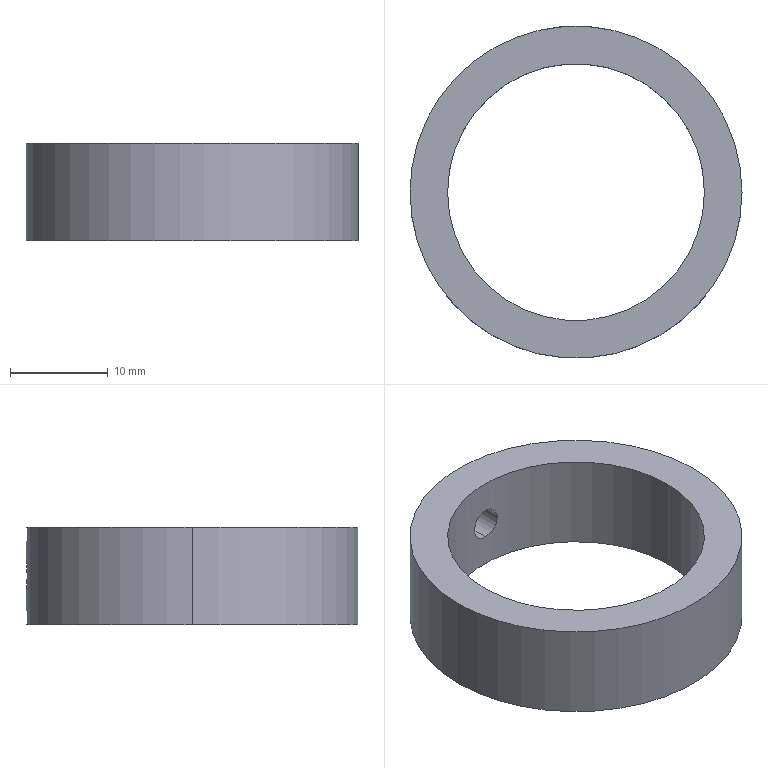Part | SolidWorks | features Extrusion 1, HoleWzd 1 | 1 solid | 8 faces | box 34 x 34 x 10 mm | volume 3614 mm3 | cylinder 6 | plane 2 | commonest cylinder face diameters 3.3 x2 26.3 x2 34 x2
STEP:
#1=CARTESIAN_POINT('',(0.,17.,1.65));
#2=VERTEX_POINT('',#1);
#3=CARTESIAN_POINT('',(0.,17.,-1.65));
#4=VERTEX_POINT('',#3);
#5=CARTESIAN_POINT('',(0.,17.,1.65));
#6=CARTESIAN_POINT('',(-0.2154,17.,1.65));
#7=CARTESIAN_POINT('',(-0.4326,16.996,1.607));
#8=CARTESIAN_POINT('',(-0.8297,16.981,1.442));
#9=CARTESIAN_POINT('',(-1.014,16.97,1.32));
#10=CARTESIAN_POINT('',(-1.242,16.955,1.092));
#11=CARTESIAN_POINT('',(-1.312,16.949,1.007));
#12=CARTESIAN_POINT('',(-1.432,16.94,0.8275));
#13=CARTESIAN_POINT('',(-1.482,16.935,0.7328));
#14=CARTESIAN_POINT('',(-1.565,16.928,0.5332));
#15=CARTESIAN_POINT('',(-1.597,16.925,0.4284));
#16=CARTESIAN_POINT('',(-1.639,16.921,0.2174));
#17=CARTESIAN_POINT('',(-1.65,16.92,0.1103));
#18=CARTESIAN_POINT('',(-1.65,16.92,-0.1077));
#19=CARTESIAN_POINT('',(-1.639,16.921,-0.2151));
#20=CARTESIAN_POINT('',(-1.598,16.925,-0.4261));
#21=CARTESIAN_POINT('',(-1.566,16.928,-0.5309));
#22=CARTESIAN_POINT('',(-1.483,16.935,-0.7308));
#23=CARTESIAN_POINT('',(-1.433,16.94,-0.8255));
#24=CARTESIAN_POINT('',(-1.313,16.949,-1.005));
#25=CARTESIAN_POINT('',(-1.244,16.955,-1.09));
#26=CARTESIAN_POINT('',(-1.016,16.97,-1.318));
#27=CARTESIAN_POINT('',(-0.8317,16.981,-1.441));
#28=CARTESIAN_POINT('',(-0.4348,16.996,-1.606));
#29=CARTESIAN_POINT('',(-0.2181,17.,-1.65));
#30=CARTESIAN_POINT('',(0.,17.,-1.65));
#31=B_SPLINE_CURVE_WITH_KNOTS('',3,(#5,#6,#7,#8,#9,#10,#11,#12,#13,#14,#15,#16,#17,#18,#19,#20,#21,#22,#23,#24,#25,#26,#27,#28,#29,#30),.UNSPECIFIED.,.F.,.F.,(4,2,2,2,2,2,2,2,2,2,2,2,4),(0.005162,0.005807,0.006452,0.006774,0.007097,0.007419,0.007742,0.008064,0.008387,0.00871,0.009032,0.009677,0.01032),.UNSPECIFIED.);
#32=EDGE_CURVE('',#2,#4,#31,.T.);
#33=ORIENTED_EDGE('',*,*,#32,.F.);
#34=CARTESIAN_POINT('',(0.,13.15,1.65));
#35=VERTEX_POINT('',#34);
#36=CARTESIAN_POINT('',(0.,0.,1.65));
#37=DIRECTION('',(0.,-1.,0.));
#38=VECTOR('',#37,1000.);
#39=LINE('',#36,#38);
#40=EDGE_CURVE('',#2,#35,#39,.T.);
#41=ORIENTED_EDGE('',*,*,#40,.T.);
#42=CARTESIAN_POINT('',(0.,13.15,-1.65));
#43=VERTEX_POINT('',#42);
#44=CARTESIAN_POINT('',(0.,13.15,1.65));
#45=CARTESIAN_POINT('',(-0.2154,13.15,1.65));
#46=CARTESIAN_POINT('',(-0.4327,13.144,1.607));
#47=CARTESIAN_POINT('',(-0.8299,13.125,1.442));
#48=CARTESIAN_POINT('',(-1.014,13.112,1.319));
#49=CARTESIAN_POINT('',(-1.242,13.091,1.092));
#50=CARTESIAN_POINT('',(-1.312,13.085,1.007));
#51=CARTESIAN_POINT('',(-1.431,13.072,0.8276));
#52=CARTESIAN_POINT('',(-1.482,13.066,0.733));
#53=CARTESIAN_POINT('',(-1.565,13.057,0.5333));
#54=CARTESIAN_POINT('',(-1.597,13.053,0.4285));
#55=CARTESIAN_POINT('',(-1.639,13.047,0.2176));
#56=CARTESIAN_POINT('',(-1.65,13.046,0.1103));
#57=CARTESIAN_POINT('',(-1.65,13.046,-0.1079));
#58=CARTESIAN_POINT('',(-1.639,13.047,-0.2152));
#59=CARTESIAN_POINT('',(-1.598,13.053,-0.4262));
#60=CARTESIAN_POINT('',(-1.566,13.056,-0.5311));
#61=CARTESIAN_POINT('',(-1.483,13.066,-0.7309));
#62=CARTESIAN_POINT('',(-1.433,13.072,-0.8256));
#63=CARTESIAN_POINT('',(-1.313,13.084,-1.005));
#64=CARTESIAN_POINT('',(-1.243,13.091,-1.09));
#65=CARTESIAN_POINT('',(-1.016,13.112,-1.318));
#66=CARTESIAN_POINT('',(-0.8318,13.125,-1.441));
#67=CARTESIAN_POINT('',(-0.435,13.144,-1.606));
#68=CARTESIAN_POINT('',(-0.2182,13.15,-1.65));
#69=CARTESIAN_POINT('',(0.,13.15,-1.65));
#70=B_SPLINE_CURVE_WITH_KNOTS('',3,(#44,#45,#46,#47,#48,#49,#50,#51,#52,#53,#54,#55,#56,#57,#58,#59,#60,#61,#62,#63,#64,#65,#66,#67,#68,#69),.UNSPECIFIED.,.F.,.F.,(4,2,2,2,2,2,2,2,2,2,2,2,4),(0.005164,0.005809,0.006454,0.006777,0.0071,0.007422,0.007745,0.008068,0.00839,0.008713,0.009036,0.009681,0.01033),.UNSPECIFIED.);
#71=EDGE_CURVE('',#35,#43,#70,.T.);
#72=ORIENTED_EDGE('',*,*,#71,.T.);
#73=CARTESIAN_POINT('',(0.,0.,-1.65));
#74=DIRECTION('',(0.,-1.,0.));
#75=VECTOR('',#74,1000.);
#76=LINE('',#73,#75);
#77=EDGE_CURVE('',#4,#43,#76,.T.);
#78=ORIENTED_EDGE('',*,*,#77,.F.);
#79=EDGE_LOOP('',(#33,#41,#72,#78));
#80=FACE_OUTER_BOUND('',#79,.T.);
#81=CARTESIAN_POINT('',(0.,0.,0.));
#82=DIRECTION('',(0.,-1.,0.));
#83=DIRECTION('',(0.,0.,-1.));
#84=AXIS2_PLACEMENT_3D('',#81,#82,#83);
#85=CYLINDRICAL_SURFACE('',#84,1.65);
#86=ADVANCED_FACE('',(#80),#85,.F.);
#87=CARTESIAN_POINT('',(-13.15,0.,5.));
#88=VERTEX_POINT('',#87);
#89=CARTESIAN_POINT('',(13.15,0.,5.));
#90=VERTEX_POINT('',#89);
#91=CARTESIAN_POINT('',(0.,0.,5.));
#92=DIRECTION('',(0.,0.,1.));
#93=DIRECTION('',(1.,0.,0.));
#94=AXIS2_PLACEMENT_3D('',#91,#92,#93);
#95=CIRCLE('',#94,13.15);
#96=EDGE_CURVE('',#88,#90,#95,.T.);
#97=ORIENTED_EDGE('',*,*,#96,.T.);
#98=CARTESIAN_POINT('',(13.15,0.,-5.));
#99=VERTEX_POINT('',#98);
#100=CARTESIAN_POINT('',(13.15,0.,5.));
#101=DIRECTION('',(0.,0.,-1.));
#102=VECTOR('',#101,1000.);
#103=LINE('',#100,#102);
#104=EDGE_CURVE('',#90,#99,#103,.T.);
#105=ORIENTED_EDGE('',*,*,#104,.T.);
#106=CARTESIAN_POINT('',(-13.15,0.,-5.));
#107=VERTEX_POINT('',#106);
#108=CARTESIAN_POINT('',(0.,0.,-5.));
#109=DIRECTION('',(0.,0.,1.));
#110=DIRECTION('',(1.,0.,0.));
#111=AXIS2_PLACEMENT_3D('',#108,#109,#110);
#112=CIRCLE('',#111,13.15);
#113=EDGE_CURVE('',#107,#99,#112,.T.);
#114=ORIENTED_EDGE('',*,*,#113,.F.);
#115=CARTESIAN_POINT('',(-13.15,0.,5.));
#116=DIRECTION('',(0.,0.,-1.));
#117=VECTOR('',#116,1000.);
#118=LINE('',#115,#117);
#119=EDGE_CURVE('',#88,#107,#118,.T.);
#120=ORIENTED_EDGE('',*,*,#119,.F.);
#121=EDGE_LOOP('',(#97,#105,#114,#120));
#122=FACE_OUTER_BOUND('',#121,.T.);
#123=CARTESIAN_POINT('',(0.,0.,5.));
#124=DIRECTION('',(0.,0.,-1.));
#125=DIRECTION('',(-1.,0.,0.));
#126=AXIS2_PLACEMENT_3D('',#123,#124,#125);
#127=CYLINDRICAL_SURFACE('',#126,13.15);
#128=ADVANCED_FACE('',(#122),#127,.F.);
#129=CARTESIAN_POINT('',(0.,17.,-1.65));
#130=CARTESIAN_POINT('',(0.1091,17.,-1.65));
#131=CARTESIAN_POINT('',(0.2163,16.999,-1.639));
#132=CARTESIAN_POINT('',(0.4273,16.995,-1.597));
#133=CARTESIAN_POINT('',(0.5322,16.992,-1.566));
#134=CARTESIAN_POINT('',(0.732,16.985,-1.483));
#135=CARTESIAN_POINT('',(0.8267,16.98,-1.432));
#136=CARTESIAN_POINT('',(1.006,16.97,-1.312));
#137=CARTESIAN_POINT('',(1.091,16.965,-1.243));
#138=CARTESIAN_POINT('',(1.319,16.949,-1.014));
#139=CARTESIAN_POINT('',(1.442,16.939,-0.8303));
#140=CARTESIAN_POINT('',(1.607,16.924,-0.4332));
#141=CARTESIAN_POINT('',(1.65,16.92,-0.216));
#142=CARTESIAN_POINT('',(1.65,16.92,0.1071));
#143=CARTESIAN_POINT('',(1.639,16.921,0.2165));
#144=CARTESIAN_POINT('',(1.597,16.925,0.4282));
#145=CARTESIAN_POINT('',(1.566,16.928,0.531));
#146=CARTESIAN_POINT('',(1.483,16.935,0.7309));
#147=CARTESIAN_POINT('',(1.432,16.94,0.8274));
#148=CARTESIAN_POINT('',(1.312,16.949,1.006));
#149=CARTESIAN_POINT('',(1.244,16.955,1.089));
#150=CARTESIAN_POINT('',(1.09,16.965,1.244));
#151=CARTESIAN_POINT('',(1.007,16.97,1.312));
#152=CARTESIAN_POINT('',(0.8279,16.98,1.431));
#153=CARTESIAN_POINT('',(0.7314,16.985,1.483));
#154=CARTESIAN_POINT('',(0.5316,16.992,1.566));
#155=CARTESIAN_POINT('',(0.4287,16.995,1.597));
#156=CARTESIAN_POINT('',(0.2171,16.999,1.639));
#157=CARTESIAN_POINT('',(0.1077,17.,1.65));
#158=CARTESIAN_POINT('',(0.,17.,1.65));
#159=B_SPLINE_CURVE_WITH_KNOTS('',3,(#129,#130,#131,#132,#133,#134,#135,#136,#137,#138,#139,#140,#141,#142,#143,#144,#145,#146,#147,#148,#149,#150,#151,#152,#153,#154,#155,#156,#157,#158),.UNSPECIFIED.,.F.,.F.,(4,2,2,2,2,2,2,2,2,2,2,2,2,2,4),(0.,0.0003226,0.0006452,0.0009678,0.00129,0.001936,0.002581,0.002903,0.003226,0.003549,0.003871,0.004194,0.004516,0.004839,0.005162),.UNSPECIFIED.);
#160=EDGE_CURVE('',#4,#2,#159,.T.);
#161=ORIENTED_EDGE('',*,*,#160,.T.);
#162=ORIENTED_EDGE('',*,*,#32,.T.);
#163=EDGE_LOOP('',(#161,#162));
#164=FACE_BOUND('',#163,.T.);
#165=CARTESIAN_POINT('',(17.,0.,5.));
#166=VERTEX_POINT('',#165);
#167=CARTESIAN_POINT('',(-17.,0.,5.));
#168=VERTEX_POINT('',#167);
#169=CARTESIAN_POINT('',(0.,0.,5.));
#170=DIRECTION('',(0.,0.,1.));
#171=DIRECTION('',(1.,0.,0.));
#172=AXIS2_PLACEMENT_3D('',#169,#170,#171);
#173=CIRCLE('',#172,17.);
#174=EDGE_CURVE('',#166,#168,#173,.T.);
#175=ORIENTED_EDGE('',*,*,#174,.F.);
#176=CARTESIAN_POINT('',(17.,0.,-5.));
#177=VERTEX_POINT('',#176);
#178=CARTESIAN_POINT('',(17.,0.,5.));
#179=DIRECTION('',(0.,0.,-1.));
#180=VECTOR('',#179,1000.);
#181=LINE('',#178,#180);
#182=EDGE_CURVE('',#166,#177,#181,.T.);
#183=ORIENTED_EDGE('',*,*,#182,.T.);
#184=CARTESIAN_POINT('',(-17.,0.,-5.));
#185=VERTEX_POINT('',#184);
#186=CARTESIAN_POINT('',(0.,0.,-5.));
#187=DIRECTION('',(0.,0.,1.));
#188=DIRECTION('',(1.,0.,0.));
#189=AXIS2_PLACEMENT_3D('',#186,#187,#188);
#190=CIRCLE('',#189,17.);
#191=EDGE_CURVE('',#177,#185,#190,.T.);
#192=ORIENTED_EDGE('',*,*,#191,.T.);
#193=CARTESIAN_POINT('',(-17.,0.,5.));
#194=DIRECTION('',(0.,0.,-1.));
#195=VECTOR('',#194,1000.);
#196=LINE('',#193,#195);
#197=EDGE_CURVE('',#168,#185,#196,.T.);
#198=ORIENTED_EDGE('',*,*,#197,.F.);
#199=EDGE_LOOP('',(#175,#183,#192,#198));
#200=FACE_OUTER_BOUND('',#199,.T.);
#201=CARTESIAN_POINT('',(0.,0.,5.));
#202=DIRECTION('',(0.,0.,-1.));
#203=DIRECTION('',(-1.,0.,0.));
#204=AXIS2_PLACEMENT_3D('',#201,#202,#203);
#205=CYLINDRICAL_SURFACE('',#204,17.);
#206=ADVANCED_FACE('',(#164,#200),#205,.T.);
#207=CARTESIAN_POINT('',(0.,0.,5.));
#208=DIRECTION('',(0.,0.,1.));
#209=DIRECTION('',(1.,0.,0.));
#210=AXIS2_PLACEMENT_3D('',#207,#208,#209);
#211=CIRCLE('',#210,17.);
#212=EDGE_CURVE('',#168,#166,#211,.T.);
#213=ORIENTED_EDGE('',*,*,#212,.T.);
#214=ORIENTED_EDGE('',*,*,#174,.T.);
#215=EDGE_LOOP('',(#213,#214));
#216=FACE_OUTER_BOUND('',#215,.T.);
#217=ORIENTED_EDGE('',*,*,#96,.F.);
#218=CARTESIAN_POINT('',(0.,0.,5.));
#219=DIRECTION('',(0.,0.,1.));
#220=DIRECTION('',(1.,0.,0.));
#221=AXIS2_PLACEMENT_3D('',#218,#219,#220);
#222=CIRCLE('',#221,13.15);
#223=EDGE_CURVE('',#90,#88,#222,.T.);
#224=ORIENTED_EDGE('',*,*,#223,.F.);
#225=EDGE_LOOP('',(#217,#224));
#226=FACE_BOUND('',#225,.T.);
#227=CARTESIAN_POINT('',(0.,0.,5.));
#228=DIRECTION('',(0.,0.,1.));
#229=DIRECTION('',(1.,0.,0.));
#230=AXIS2_PLACEMENT_3D('',#227,#228,#229);
#231=PLANE('',#230);
#232=ADVANCED_FACE('',(#216,#226),#231,.T.);
#233=CARTESIAN_POINT('',(0.,0.,-5.));
#234=DIRECTION('',(0.,0.,1.));
#235=DIRECTION('',(1.,0.,0.));
#236=AXIS2_PLACEMENT_3D('',#233,#234,#235);
#237=CIRCLE('',#236,17.);
#238=EDGE_CURVE('',#185,#177,#237,.T.);
#239=ORIENTED_EDGE('',*,*,#238,.F.);
#240=ORIENTED_EDGE('',*,*,#191,.F.);
#241=EDGE_LOOP('',(#239,#240));
#242=FACE_OUTER_BOUND('',#241,.T.);
#243=ORIENTED_EDGE('',*,*,#113,.T.);
#244=CARTESIAN_POINT('',(0.,0.,-5.));
#245=DIRECTION('',(0.,0.,1.));
#246=DIRECTION('',(1.,0.,0.));
#247=AXIS2_PLACEMENT_3D('',#244,#245,#246);
#248=CIRCLE('',#247,13.15);
#249=EDGE_CURVE('',#99,#107,#248,.T.);
#250=ORIENTED_EDGE('',*,*,#249,.T.);
#251=EDGE_LOOP('',(#243,#250));
#252=FACE_BOUND('',#251,.T.);
#253=CARTESIAN_POINT('',(0.,0.,-5.));
#254=DIRECTION('',(0.,0.,1.));
#255=DIRECTION('',(1.,0.,0.));
#256=AXIS2_PLACEMENT_3D('',#253,#254,#255);
#257=PLANE('',#256);
#258=ADVANCED_FACE('',(#242,#252),#257,.F.);
#259=ORIENTED_EDGE('',*,*,#182,.F.);
#260=ORIENTED_EDGE('',*,*,#212,.F.);
#261=ORIENTED_EDGE('',*,*,#197,.T.);
#262=ORIENTED_EDGE('',*,*,#238,.T.);
#263=EDGE_LOOP('',(#259,#260,#261,#262));
#264=FACE_OUTER_BOUND('',#263,.T.);
#265=CARTESIAN_POINT('',(0.,0.,5.));
#266=DIRECTION('',(0.,0.,-1.));
#267=DIRECTION('',(-1.,0.,0.));
#268=AXIS2_PLACEMENT_3D('',#265,#266,#267);
#269=CYLINDRICAL_SURFACE('',#268,17.);
#270=ADVANCED_FACE('',(#264),#269,.T.);
#271=ORIENTED_EDGE('',*,*,#104,.F.);
#272=ORIENTED_EDGE('',*,*,#223,.T.);
#273=ORIENTED_EDGE('',*,*,#119,.T.);
#274=ORIENTED_EDGE('',*,*,#249,.F.);
#275=EDGE_LOOP('',(#271,#272,#273,#274));
#276=FACE_OUTER_BOUND('',#275,.T.);
#277=CARTESIAN_POINT('',(0.,13.15,-1.65));
#278=CARTESIAN_POINT('',(0.1091,13.15,-1.65));
#279=CARTESIAN_POINT('',(0.2164,13.149,-1.639));
#280=CARTESIAN_POINT('',(0.4275,13.143,-1.597));
#281=CARTESIAN_POINT('',(0.5323,13.14,-1.566));
#282=CARTESIAN_POINT('',(0.7321,13.13,-1.483));
#283=CARTESIAN_POINT('',(0.8269,13.124,-1.432));
#284=CARTESIAN_POINT('',(1.006,13.112,-1.312));
#285=CARTESIAN_POINT('',(1.091,13.105,-1.243));
#286=CARTESIAN_POINT('',(1.319,13.085,-1.014));
#287=CARTESIAN_POINT('',(1.442,13.071,-0.8304));
#288=CARTESIAN_POINT('',(1.607,13.052,-0.4334));
#289=CARTESIAN_POINT('',(1.65,13.046,-0.2161));
#290=CARTESIAN_POINT('',(1.65,13.046,0.1071));
#291=CARTESIAN_POINT('',(1.639,13.047,0.2166));
#292=CARTESIAN_POINT('',(1.597,13.053,0.4283));
#293=CARTESIAN_POINT('',(1.566,13.057,0.5312));
#294=CARTESIAN_POINT('',(1.483,13.066,0.7311));
#295=CARTESIAN_POINT('',(1.431,13.072,0.8276));
#296=CARTESIAN_POINT('',(1.312,13.085,1.006));
#297=CARTESIAN_POINT('',(1.244,13.091,1.09));
#298=CARTESIAN_POINT('',(1.09,13.105,1.244));
#299=CARTESIAN_POINT('',(1.007,13.112,1.312));
#300=CARTESIAN_POINT('',(0.828,13.124,1.431));
#301=CARTESIAN_POINT('',(0.7315,13.13,1.483));
#302=CARTESIAN_POINT('',(0.5317,13.14,1.566));
#303=CARTESIAN_POINT('',(0.4289,13.143,1.597));
#304=CARTESIAN_POINT('',(0.2172,13.149,1.639));
#305=CARTESIAN_POINT('',(0.1077,13.15,1.65));
#306=CARTESIAN_POINT('',(0.,13.15,1.65));
#307=B_SPLINE_CURVE_WITH_KNOTS('',3,(#277,#278,#279,#280,#281,#282,#283,#284,#285,#286,#287,#288,#289,#290,#291,#292,#293,#294,#295,#296,#297,#298,#299,#300,#301,#302,#303,#304,#305,#306),.UNSPECIFIED.,.F.,.F.,(4,2,2,2,2,2,2,2,2,2,2,2,2,2,4),(0.,0.0003227,0.0006455,0.0009682,0.001291,0.001936,0.002582,0.002905,0.003227,0.00355,0.003873,0.004196,0.004518,0.004841,0.005164),.UNSPECIFIED.);
#308=EDGE_CURVE('',#43,#35,#307,.T.);
#309=ORIENTED_EDGE('',*,*,#308,.F.);
#310=ORIENTED_EDGE('',*,*,#71,.F.);
#311=EDGE_LOOP('',(#309,#310));
#312=FACE_BOUND('',#311,.T.);
#313=CARTESIAN_POINT('',(0.,0.,5.));
#314=DIRECTION('',(0.,0.,-1.));
#315=DIRECTION('',(-1.,0.,0.));
#316=AXIS2_PLACEMENT_3D('',#313,#314,#315);
#317=CYLINDRICAL_SURFACE('',#316,13.15);
#318=ADVANCED_FACE('',(#276,#312),#317,.F.);
#319=ORIENTED_EDGE('',*,*,#40,.F.);
#320=ORIENTED_EDGE('',*,*,#160,.F.);
#321=ORIENTED_EDGE('',*,*,#77,.T.);
#322=ORIENTED_EDGE('',*,*,#308,.T.);
#323=EDGE_LOOP('',(#319,#320,#321,#322));
#324=FACE_OUTER_BOUND('',#323,.T.);
#325=CARTESIAN_POINT('',(0.,0.,0.));
#326=DIRECTION('',(0.,-1.,0.));
#327=DIRECTION('',(0.,0.,-1.));
#328=AXIS2_PLACEMENT_3D('',#325,#326,#327);
#329=CYLINDRICAL_SURFACE('',#328,1.65);
#330=ADVANCED_FACE('',(#324),#329,.F.);
#331=CLOSED_SHELL('',(#86,#128,#206,#232,#258,#270,#318,#330));
#332=MANIFOLD_SOLID_BREP('',#331);
#333=CARTESIAN_POINT('',(0.,0.,0.));
#334=DIRECTION('',(0.,0.,1.));
#335=DIRECTION('',(1.,0.,0.));
#336=AXIS2_PLACEMENT_3D('',#333,#334,#335);
#337=(LENGTH_UNIT()NAMED_UNIT(*)SI_UNIT(.MILLI.,.METRE.));
#338=UNCERTAINTY_MEASURE_WITH_UNIT(LENGTH_MEASURE(0.00001),#337,'','');
#339=(NAMED_UNIT(*)PLANE_ANGLE_UNIT()SI_UNIT($,.RADIAN.));
#340=(NAMED_UNIT(*)SI_UNIT($,.STERADIAN.)SOLID_ANGLE_UNIT());
#341=(GEOMETRIC_REPRESENTATION_CONTEXT(3)GLOBAL_UNCERTAINTY_ASSIGNED_CONTEXT((#338))GLOBAL_UNIT_ASSIGNED_CONTEXT((#337,#339,#340))REPRESENTATION_CONTEXT('',''));
#342=ADVANCED_BREP_SHAPE_REPRESENTATION('',(#332,#336),#341);